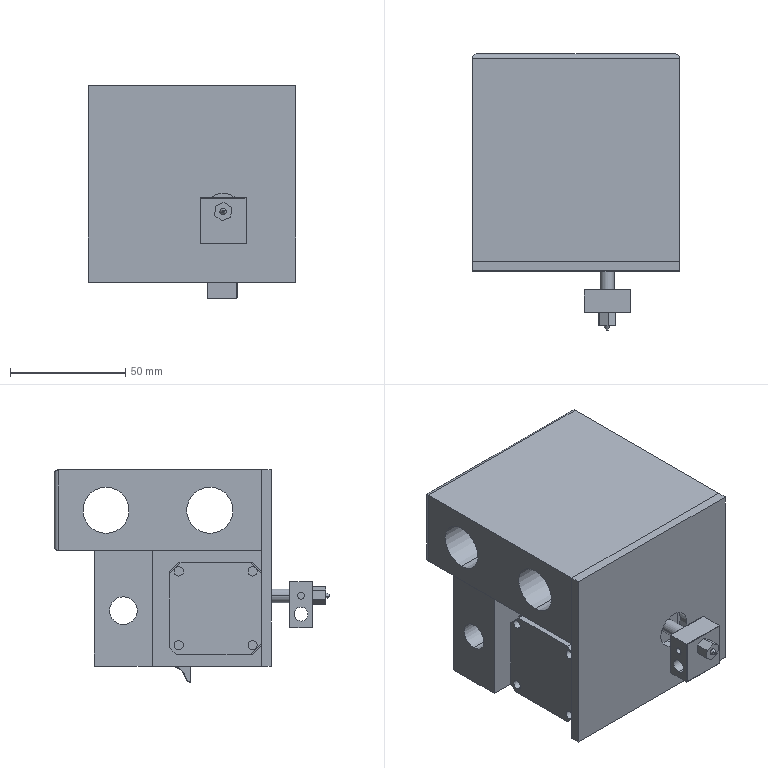Part | SolidWorks | features InContextFeatHolder 2 | 30 solids | 1072 faces | box 90 x 119.5 x 91.979 mm | volume 440210 mm3 | cylinder 406 | plane 400 | cone 116 | spline 74 | torus 66 | sphere 10 | commonest cylinder face diameters 1 x73 4 x45 11 x42 5 x32 24 x28 8 x26